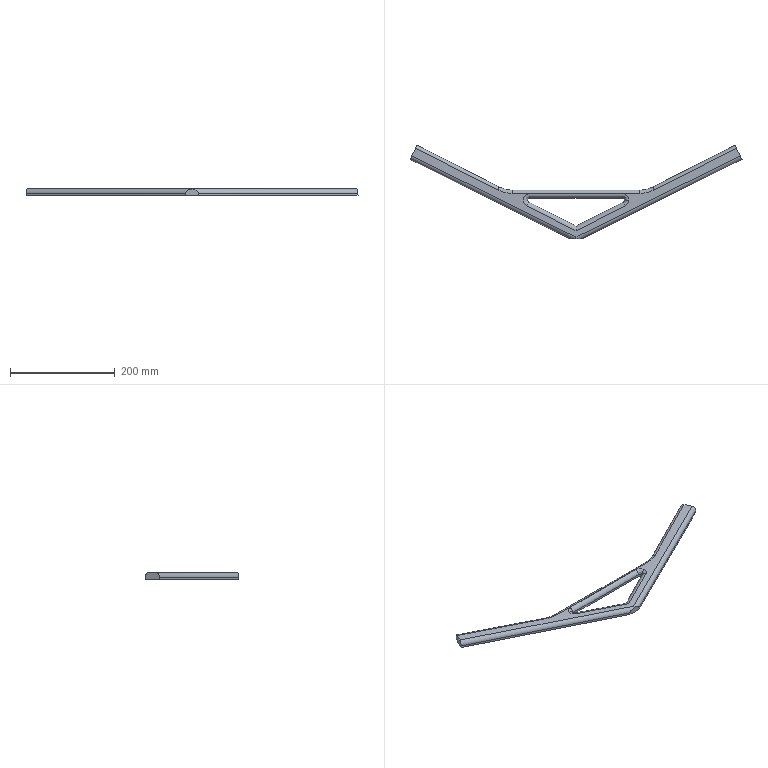Part | SolidWorks | features BaseBody 1 | 1 solid | 31 faces | box 633.433 x 177.606 x 12 mm | volume 259500 mm3 | cylinder 13 | plane 13 | spline 5 | commonest cylinder face diameters 16 x5 8 x3 12 x3 108 x2
STEP:
#1=CARTESIAN_POINT('',(-92.659,64.368,4.));
#2=VERTEX_POINT('',#1);
#3=CARTESIAN_POINT('',(-88.659,68.368,4.));
#4=VERTEX_POINT('',#3);
#5=CARTESIAN_POINT('',(-88.659,64.368,4.));
#6=DIRECTION('',(0.,0.,-1.));
#7=DIRECTION('',(-1.,0.,0.));
#8=AXIS2_PLACEMENT_3D('',#5,#6,#7);
#9=CIRCLE('',#8,4.);
#10=EDGE_CURVE('',#2,#4,#9,.T.);
#11=ORIENTED_EDGE('',*,*,#10,.F.);
#12=CARTESIAN_POINT('',(-92.659,64.368,0.));
#13=VERTEX_POINT('',#12);
#14=CARTESIAN_POINT('',(-92.659,64.368,4.));
#15=DIRECTION('',(0.,0.,-1.));
#16=VECTOR('',#15,1000.);
#17=LINE('',#14,#16);
#18=EDGE_CURVE('',#2,#13,#17,.T.);
#19=ORIENTED_EDGE('',*,*,#18,.T.);
#20=CARTESIAN_POINT('',(-88.659,68.368,0.));
#21=VERTEX_POINT('',#20);
#22=CARTESIAN_POINT('',(-88.659,64.368,0.));
#23=DIRECTION('',(0.,0.,-1.));
#24=DIRECTION('',(-1.,0.,0.));
#25=AXIS2_PLACEMENT_3D('',#22,#23,#24);
#26=CIRCLE('',#25,4.);
#27=EDGE_CURVE('',#13,#21,#26,.T.);
#28=ORIENTED_EDGE('',*,*,#27,.T.);
#29=CARTESIAN_POINT('',(-88.659,68.368,2.));
#30=DIRECTION('',(0.,0.,-1.));
#31=VECTOR('',#30,1000.);
#32=LINE('',#29,#31);
#33=EDGE_CURVE('',#4,#21,#32,.T.);
#34=ORIENTED_EDGE('',*,*,#33,.F.);
#35=EDGE_LOOP('',(#11,#19,#28,#34));
#36=FACE_OUTER_BOUND('',#35,.T.);
#37=CARTESIAN_POINT('',(-88.659,64.368,4.));
#38=DIRECTION('',(0.,0.,-1.));
#39=DIRECTION('',(-1.,0.,0.));
#40=AXIS2_PLACEMENT_3D('',#37,#38,#39);
#41=CYLINDRICAL_SURFACE('',#40,4.);
#42=ADVANCED_FACE('',(#36),#41,.F.);
#43=CARTESIAN_POINT('',(92.659,64.368,4.));
#44=VERTEX_POINT('',#43);
#45=CARTESIAN_POINT('',(90.467,60.8,4.));
#46=VERTEX_POINT('',#45);
#47=CARTESIAN_POINT('',(88.659,64.368,4.));
#48=DIRECTION('',(0.,0.,-1.));
#49=DIRECTION('',(-1.,0.,0.));
#50=AXIS2_PLACEMENT_3D('',#47,#48,#49);
#51=CIRCLE('',#50,4.);
#52=EDGE_CURVE('',#44,#46,#51,.T.);
#53=ORIENTED_EDGE('',*,*,#52,.T.);
#54=CARTESIAN_POINT('',(94.083,53.664,12.));
#55=VERTEX_POINT('',#54);
#56=CARTESIAN_POINT('',(94.083,53.664,4.));
#57=DIRECTION('',(0.892,0.452,0.));
#58=DIRECTION('',(-0.452,0.892,0.));
#59=AXIS2_PLACEMENT_3D('',#56,#57,#58);
#60=CIRCLE('',#59,8.);
#61=EDGE_CURVE('',#46,#55,#60,.T.);
#62=ORIENTED_EDGE('',*,*,#61,.T.);
#63=CARTESIAN_POINT('',(100.659,64.368,12.));
#64=VERTEX_POINT('',#63);
#65=CARTESIAN_POINT('',(94.083,53.664,12.));
#66=CARTESIAN_POINT('',(98.227,55.764,12.));
#67=CARTESIAN_POINT('',(100.659,59.722,12.));
#68=CARTESIAN_POINT('',(100.659,64.368,12.));
#69=(BOUNDED_CURVE()B_SPLINE_CURVE(3,(#65,#66,#67,#68),.UNSPECIFIED.,.F.,.F.)B_SPLINE_CURVE_WITH_KNOTS((4,4),(0.,1.),.UNSPECIFIED.)CURVE()GEOMETRIC_REPRESENTATION_ITEM()RATIONAL_B_SPLINE_CURVE((0.9566,0.8622,0.8622,0.9566))REPRESENTATION_ITEM(''));
#70=EDGE_CURVE('',#55,#64,#69,.T.);
#71=ORIENTED_EDGE('',*,*,#70,.T.);
#72=CARTESIAN_POINT('',(100.659,64.368,12.));
#73=CARTESIAN_POINT('',(95.973,64.368,12.));
#74=CARTESIAN_POINT('',(92.659,64.368,8.686));
#75=CARTESIAN_POINT('',(92.659,64.368,4.));
#76=(BOUNDED_CURVE()B_SPLINE_CURVE(3,(#72,#73,#74,#75),.UNSPECIFIED.,.F.,.F.)B_SPLINE_CURVE_WITH_KNOTS((4,4),(0.06314,0.9369),.UNSPECIFIED.)CURVE()GEOMETRIC_REPRESENTATION_ITEM()RATIONAL_B_SPLINE_CURVE((0.9566,0.7698,0.7698,0.9566))REPRESENTATION_ITEM(''));
#77=EDGE_CURVE('',#64,#44,#76,.T.);
#78=ORIENTED_EDGE('',*,*,#77,.T.);
#79=EDGE_LOOP('',(#53,#62,#71,#78));
#80=FACE_OUTER_BOUND('',#79,.T.);
#81=CARTESIAN_POINT('',(90.485,60.764,3.201));
#82=CARTESIAN_POINT('',(91.88,61.471,3.201));
#83=CARTESIAN_POINT('',(92.699,62.804,3.201));
#84=CARTESIAN_POINT('',(92.699,64.368,3.201));
#85=CARTESIAN_POINT('',(90.238,61.251,8.64));
#86=CARTESIAN_POINT('',(91.445,61.862,8.64));
#87=CARTESIAN_POINT('',(92.153,63.015,8.64));
#88=CARTESIAN_POINT('',(92.153,64.368,8.64));
#89=CARTESIAN_POINT('',(91.986,57.803,12.506));
#90=CARTESIAN_POINT('',(94.527,59.091,12.506));
#91=CARTESIAN_POINT('',(96.018,61.518,12.506));
#92=CARTESIAN_POINT('',(96.018,64.368,12.506));
#93=CARTESIAN_POINT('',(94.444,52.951,11.96));
#94=CARTESIAN_POINT('',(98.864,55.191,11.96));
#95=CARTESIAN_POINT('',(101.458,59.413,11.96));
#96=CARTESIAN_POINT('',(101.458,64.368,11.96));
#97=(BOUNDED_SURFACE()B_SPLINE_SURFACE(3,3,((#81,#82,#83,#84),(#85,#86,#87,#88),(#89,#90,#91,#92),(#93,#94,#95,#96)),.UNSPECIFIED.,.F.,.F.,.T.)B_SPLINE_SURFACE_WITH_KNOTS((4,4),(4,4),(0.,1.),(0.,1.),.UNSPECIFIED.)GEOMETRIC_REPRESENTATION_ITEM()RATIONAL_B_SPLINE_SURFACE(((1.,0.9014,0.9014,1.),(0.7553,0.6808,0.6808,0.7553),(0.7553,0.6808,0.6808,0.7553),(1.,0.9014,0.9014,1.)))REPRESENTATION_ITEM('')SURFACE());
#98=ADVANCED_FACE('',(#80),#97,.T.);
#99=CARTESIAN_POINT('',(0.,14.953,4.));
#100=VERTEX_POINT('',#99);
#101=CARTESIAN_POINT('',(43.143,36.817,4.));
#102=DIRECTION('',(0.892,0.452,0.));
#103=VECTOR('',#102,1000.);
#104=LINE('',#101,#103);
#105=EDGE_CURVE('',#100,#46,#104,.T.);
#106=ORIENTED_EDGE('',*,*,#105,.F.);
#107=CARTESIAN_POINT('',(0.000000027,5.985,12.));
#108=VERTEX_POINT('',#107);
#109=CARTESIAN_POINT('',(0.000000027,5.985,12.));
#110=CARTESIAN_POINT('',(0.,11.239,12.));
#111=CARTESIAN_POINT('',(0.,14.953,8.686));
#112=CARTESIAN_POINT('',(0.,14.953,4.));
#113=(BOUNDED_CURVE()B_SPLINE_CURVE(3,(#109,#110,#111,#112),.UNSPECIFIED.,.F.,.F.)B_SPLINE_CURVE_WITH_KNOTS((4,4),(4.712,6.283),.UNSPECIFIED.)CURVE()GEOMETRIC_REPRESENTATION_ITEM()RATIONAL_B_SPLINE_CURVE((1.,0.8047,0.8047,1.))REPRESENTATION_ITEM(''));
#114=EDGE_CURVE('',#108,#100,#113,.T.);
#115=ORIENTED_EDGE('',*,*,#114,.F.);
#116=CARTESIAN_POINT('',(46.759,29.681,12.));
#117=DIRECTION('',(-0.892,-0.452,0.));
#118=VECTOR('',#117,1000.);
#119=LINE('',#116,#118);
#120=EDGE_CURVE('',#55,#108,#119,.T.);
#121=ORIENTED_EDGE('',*,*,#120,.F.);
#122=ORIENTED_EDGE('',*,*,#61,.F.);
#123=EDGE_LOOP('',(#106,#115,#121,#122));
#124=FACE_OUTER_BOUND('',#123,.T.);
#125=CARTESIAN_POINT('',(-0.5645,5.699,4.));
#126=DIRECTION('',(0.892,0.452,0.));
#127=DIRECTION('',(-0.452,0.892,0.));
#128=AXIS2_PLACEMENT_3D('',#125,#126,#127);
#129=CYLINDRICAL_SURFACE('',#128,8.);
#130=ADVANCED_FACE('',(#124),#129,.T.);
#131=CARTESIAN_POINT('',(88.659,68.368,4.));
#132=VERTEX_POINT('',#131);
#133=CARTESIAN_POINT('',(88.659,68.368,0.));
#134=VERTEX_POINT('',#133);
#135=CARTESIAN_POINT('',(88.659,68.368,2.));
#136=DIRECTION('',(0.,0.,-1.));
#137=VECTOR('',#136,1000.);
#138=LINE('',#135,#137);
#139=EDGE_CURVE('',#132,#134,#138,.T.);
#140=ORIENTED_EDGE('',*,*,#139,.T.);
#141=CARTESIAN_POINT('',(90.467,60.8,0.));
#142=VERTEX_POINT('',#141);
#143=CARTESIAN_POINT('',(88.659,64.368,0.));
#144=DIRECTION('',(0.,0.,-1.));
#145=DIRECTION('',(-1.,0.,0.));
#146=AXIS2_PLACEMENT_3D('',#143,#144,#145);
#147=CIRCLE('',#146,4.);
#148=EDGE_CURVE('',#134,#142,#147,.T.);
#149=ORIENTED_EDGE('',*,*,#148,.T.);
#150=CARTESIAN_POINT('',(90.467,60.8,2.));
#151=DIRECTION('',(0.,0.,1.));
#152=VECTOR('',#151,1000.);
#153=LINE('',#150,#152);
#154=EDGE_CURVE('',#142,#46,#153,.T.);
#155=ORIENTED_EDGE('',*,*,#154,.T.);
#156=ORIENTED_EDGE('',*,*,#52,.F.);
#157=CARTESIAN_POINT('',(88.659,64.368,4.));
#158=DIRECTION('',(0.,0.,1.));
#159=DIRECTION('',(-1.,0.,0.));
#160=AXIS2_PLACEMENT_3D('',#157,#158,#159);
#161=CIRCLE('',#160,4.);
#162=EDGE_CURVE('',#44,#132,#161,.T.);
#163=ORIENTED_EDGE('',*,*,#162,.T.);
#164=EDGE_LOOP('',(#140,#149,#155,#156,#163));
#165=FACE_OUTER_BOUND('',#164,.T.);
#166=CARTESIAN_POINT('',(88.659,64.368,4.));
#167=DIRECTION('',(0.,0.,-1.));
#168=DIRECTION('',(-1.,0.,0.));
#169=AXIS2_PLACEMENT_3D('',#166,#167,#168);
#170=CYLINDRICAL_SURFACE('',#169,4.);
#171=ADVANCED_FACE('',(#165),#170,.F.);
#172=CARTESIAN_POINT('',(88.659,76.368,12.));
#173=VERTEX_POINT('',#172);
#174=CARTESIAN_POINT('',(88.659,76.368,4.));
#175=DIRECTION('',(1.,0.,0.));
#176=DIRECTION('',(0.,0.,-1.));
#177=AXIS2_PLACEMENT_3D('',#174,#175,#176);
#178=CIRCLE('',#177,8.);
#179=EDGE_CURVE('',#173,#132,#178,.T.);
#180=ORIENTED_EDGE('',*,*,#179,.T.);
#181=ORIENTED_EDGE('',*,*,#162,.F.);
#182=ORIENTED_EDGE('',*,*,#77,.F.);
#183=CARTESIAN_POINT('',(100.659,64.368,12.));
#184=CARTESIAN_POINT('',(100.659,71.397,12.));
#185=CARTESIAN_POINT('',(95.688,76.368,12.));
#186=CARTESIAN_POINT('',(88.659,76.368,12.));
#187=(BOUNDED_CURVE()B_SPLINE_CURVE(3,(#183,#184,#185,#186),.UNSPECIFIED.,.F.,.F.)B_SPLINE_CURVE_WITH_KNOTS((4,4),(0.,1.),.UNSPECIFIED.)CURVE()GEOMETRIC_REPRESENTATION_ITEM()RATIONAL_B_SPLINE_CURVE((0.9566,0.7698,0.7698,0.9566))REPRESENTATION_ITEM(''));
#188=EDGE_CURVE('',#64,#173,#187,.T.);
#189=ORIENTED_EDGE('',*,*,#188,.T.);
#190=EDGE_LOOP('',(#180,#181,#182,#189));
#191=FACE_OUTER_BOUND('',#190,.T.);
#192=CARTESIAN_POINT('',(92.699,64.368,3.201));
#193=CARTESIAN_POINT('',(92.699,66.734,3.201));
#194=CARTESIAN_POINT('',(91.025,68.408,3.201));
#195=CARTESIAN_POINT('',(88.659,68.408,3.201));
#196=CARTESIAN_POINT('',(92.153,64.368,8.64));
#197=CARTESIAN_POINT('',(92.153,66.414,8.64));
#198=CARTESIAN_POINT('',(90.706,67.862,8.64));
#199=CARTESIAN_POINT('',(88.659,67.862,8.64));
#200=CARTESIAN_POINT('',(96.018,64.368,12.506));
#201=CARTESIAN_POINT('',(96.018,68.679,12.506));
#202=CARTESIAN_POINT('',(92.97,71.727,12.506));
#203=CARTESIAN_POINT('',(88.659,71.727,12.506));
#204=CARTESIAN_POINT('',(101.458,64.368,11.96));
#205=CARTESIAN_POINT('',(101.458,71.865,11.96));
#206=CARTESIAN_POINT('',(96.156,77.166,11.96));
#207=CARTESIAN_POINT('',(88.659,77.166,11.96));
#208=(BOUNDED_SURFACE()B_SPLINE_SURFACE(3,3,((#192,#193,#194,#195),(#196,#197,#198,#199),(#200,#201,#202,#203),(#204,#205,#206,#207)),.UNSPECIFIED.,.F.,.F.,.F.)B_SPLINE_SURFACE_WITH_KNOTS((4,4),(4,4),(0.,1.),(0.,1.),.UNSPECIFIED.)GEOMETRIC_REPRESENTATION_ITEM()RATIONAL_B_SPLINE_SURFACE(((1.,0.8047,0.8047,1.),(0.7553,0.6078,0.6078,0.7553),(0.7553,0.6078,0.6078,0.7553),(1.,0.8047,0.8047,1.)))REPRESENTATION_ITEM('')SURFACE());
#209=ADVANCED_FACE('',(#191),#208,.T.);
#210=ORIENTED_EDGE('',*,*,#188,.F.);
#211=ORIENTED_EDGE('',*,*,#70,.F.);
#212=ORIENTED_EDGE('',*,*,#120,.T.);
#213=CARTESIAN_POINT('',(-94.083,53.664,12.));
#214=VERTEX_POINT('',#213);
#215=CARTESIAN_POINT('',(0.000000106,5.985,12.));
#216=DIRECTION('',(-0.892,0.452,0.));
#217=VECTOR('',#216,1000.);
#218=LINE('',#215,#217);
#219=EDGE_CURVE('',#108,#214,#218,.T.);
#220=ORIENTED_EDGE('',*,*,#219,.T.);
#221=CARTESIAN_POINT('',(-88.659,76.368,12.));
#222=VERTEX_POINT('',#221);
#223=CARTESIAN_POINT('',(-94.083,53.664,12.));
#224=CARTESIAN_POINT('',(-94.311,53.779,12.));
#225=CARTESIAN_POINT('',(-94.647,53.963,12.));
#226=CARTESIAN_POINT('',(-95.027,54.196,12.));
#227=CARTESIAN_POINT('',(-95.215,54.316,12.));
#228=CARTESIAN_POINT('',(-95.308,54.378,12.));
#229=CARTESIAN_POINT('',(-95.348,54.405,12.));
#230=CARTESIAN_POINT('',(-95.374,54.423,12.));
#231=CARTESIAN_POINT('',(-95.386,54.431,12.));
#232=CARTESIAN_POINT('',(-95.632,54.598,12.));
#233=CARTESIAN_POINT('',(-95.971,54.845,12.));
#234=CARTESIAN_POINT('',(-96.35,55.154,12.));
#235=CARTESIAN_POINT('',(-96.535,55.314,12.));
#236=CARTESIAN_POINT('',(-96.627,55.395,12.));
#237=CARTESIAN_POINT('',(-96.666,55.43,12.));
#238=CARTESIAN_POINT('',(-96.693,55.453,12.));
#239=CARTESIAN_POINT('',(-96.704,55.464,12.));
#240=CARTESIAN_POINT('',(-96.945,55.682,12.));
#241=CARTESIAN_POINT('',(-97.271,56.002,12.));
#242=CARTESIAN_POINT('',(-97.63,56.396,12.));
#243=CARTESIAN_POINT('',(-97.805,56.598,12.));
#244=CARTESIAN_POINT('',(-97.89,56.7,12.));
#245=CARTESIAN_POINT('',(-97.927,56.745,12.));
#246=CARTESIAN_POINT('',(-97.951,56.774,12.));
#247=CARTESIAN_POINT('',(-97.962,56.788,12.));
#248=CARTESIAN_POINT('',(-98.183,57.06,12.));
#249=CARTESIAN_POINT('',(-98.478,57.456,12.));
#250=CARTESIAN_POINT('',(-98.794,57.938,12.));
#251=CARTESIAN_POINT('',(-98.944,58.185,12.));
#252=CARTESIAN_POINT('',(-99.017,58.309,12.));
#253=CARTESIAN_POINT('',(-99.048,58.363,12.));
#254=CARTESIAN_POINT('',(-99.069,58.398,12.));
#255=CARTESIAN_POINT('',(-99.079,58.415,12.));
#256=CARTESIAN_POINT('',(-99.264,58.741,12.));
#257=CARTESIAN_POINT('',(-99.505,59.212,12.));
#258=CARTESIAN_POINT('',(-99.749,59.777,12.));
#259=CARTESIAN_POINT('',(-99.862,60.065,12.));
#260=CARTESIAN_POINT('',(-99.916,60.209,12.));
#261=CARTESIAN_POINT('',(-99.938,60.272,12.));
#262=CARTESIAN_POINT('',(-99.953,60.313,12.));
#263=CARTESIAN_POINT('',(-99.96,60.333,12.));
#264=CARTESIAN_POINT('',(-100.093,60.706,12.));
#265=CARTESIAN_POINT('',(-100.255,61.239,12.));
#266=CARTESIAN_POINT('',(-100.399,61.873,12.));
#267=CARTESIAN_POINT('',(-100.461,62.192,12.));
#268=CARTESIAN_POINT('',(-100.485,62.33,12.));
#269=CARTESIAN_POINT('',(-100.5,62.422,12.));
#270=CARTESIAN_POINT('',(-100.507,62.466,12.));
#271=CARTESIAN_POINT('',(-100.575,62.896,12.));
#272=CARTESIAN_POINT('',(-100.636,63.471,12.));
#273=CARTESIAN_POINT('',(-100.66,64.146,12.));
#274=CARTESIAN_POINT('',(-100.659,64.435,12.));
#275=CARTESIAN_POINT('',(-100.656,64.628,12.));
#276=CARTESIAN_POINT('',(-100.654,64.723,12.));
#277=CARTESIAN_POINT('',(-100.62,65.61,12.));
#278=CARTESIAN_POINT('',(-100.514,66.389,12.));
#279=CARTESIAN_POINT('',(-100.239,67.54,12.));
#280=CARTESIAN_POINT('',(-100.074,68.106,12.));
#281=CARTESIAN_POINT('',(-99.833,68.75,12.));
#282=CARTESIAN_POINT('',(-99.72,69.022,12.));
#283=CARTESIAN_POINT('',(-99.642,69.203,12.));
#284=CARTESIAN_POINT('',(-99.601,69.295,12.));
#285=CARTESIAN_POINT('',(-99.399,69.735,12.));
#286=CARTESIAN_POINT('',(-99.132,70.248,12.));
#287=CARTESIAN_POINT('',(-98.778,70.822,12.));
#288=CARTESIAN_POINT('',(-98.591,71.103,12.));
#289=CARTESIAN_POINT('',(-98.508,71.222,12.));
#290=CARTESIAN_POINT('',(-98.453,71.302,12.));
#291=CARTESIAN_POINT('',(-98.424,71.342,12.));
#292=CARTESIAN_POINT('',(-98.179,71.683,12.));
#293=CARTESIAN_POINT('',(-97.832,72.119,12.));
#294=CARTESIAN_POINT('',(-97.394,72.599,12.));
#295=CARTESIAN_POINT('',(-97.166,72.832,12.));
#296=CARTESIAN_POINT('',(-97.05,72.946,12.));
#297=CARTESIAN_POINT('',(-97.,72.995,12.));
#298=CARTESIAN_POINT('',(-96.966,73.027,12.));
#299=CARTESIAN_POINT('',(-96.949,73.044,12.));
#300=CARTESIAN_POINT('',(-96.677,73.303,12.));
#301=CARTESIAN_POINT('',(-96.279,73.65,12.));
#302=CARTESIAN_POINT('',(-95.788,74.023,12.));
#303=CARTESIAN_POINT('',(-95.537,74.202,12.));
#304=CARTESIAN_POINT('',(-95.409,74.289,12.));
#305=CARTESIAN_POINT('',(-95.354,74.326,12.));
#306=CARTESIAN_POINT('',(-95.318,74.351,12.));
#307=CARTESIAN_POINT('',(-95.298,74.364,12.));
#308=CARTESIAN_POINT('',(-95.006,74.557,12.));
#309=CARTESIAN_POINT('',(-94.583,74.813,12.));
#310=CARTESIAN_POINT('',(-94.072,75.08,12.));
#311=CARTESIAN_POINT('',(-93.812,75.205,12.));
#312=CARTESIAN_POINT('',(-93.681,75.266,12.));
#313=CARTESIAN_POINT('',(-93.625,75.292,12.));
#314=CARTESIAN_POINT('',(-93.587,75.309,12.));
#315=CARTESIAN_POINT('',(-93.567,75.318,12.));
#316=CARTESIAN_POINT('',(-93.271,75.45,12.));
#317=CARTESIAN_POINT('',(-92.847,75.62,12.));
#318=CARTESIAN_POINT('',(-92.341,75.79,12.));
#319=CARTESIAN_POINT('',(-92.086,75.868,12.));
#320=CARTESIAN_POINT('',(-91.958,75.905,12.));
#321=CARTESIAN_POINT('',(-91.903,75.921,12.));
#322=CARTESIAN_POINT('',(-91.866,75.931,12.));
#323=CARTESIAN_POINT('',(-91.846,75.937,12.));
#324=CARTESIAN_POINT('',(-91.559,76.015,12.));
#325=CARTESIAN_POINT('',(-91.151,76.112,12.));
#326=CARTESIAN_POINT('',(-90.67,76.199,12.));
#327=CARTESIAN_POINT('',(-90.428,76.237,12.));
#328=CARTESIAN_POINT('',(-90.307,76.254,12.));
#329=CARTESIAN_POINT('',(-90.255,76.261,12.));
#330=CARTESIAN_POINT('',(-90.22,76.266,12.));
#331=CARTESIAN_POINT('',(-90.201,76.268,12.));
#332=CARTESIAN_POINT('',(-89.679,76.335,12.));
#333=CARTESIAN_POINT('',(-89.17,76.367,12.));
#334=CARTESIAN_POINT('',(-88.659,76.368,12.));
#335=B_SPLINE_CURVE_WITH_KNOTS('',3,(#223,#224,#225,#226,#227,#228,#229,#230,#231,#232,#233,#234,#235,#236,#237,#238,#239,#240,#241,#242,#243,#244,#245,#246,#247,#248,#249,#250,#251,#252,#253,#254,#255,#256,#257,#258,#259,#260,#261,#262,#263,#264,#265,#266,#267,#268,#269,#270,#271,#272,#273,#274,#275,#276,#277,#278,#279,#280,#281,#282,#283,#284,#285,#286,#287,#288,#289,#290,#291,#292,#293,#294,#295,#296,#297,#298,#299,#300,#301,#302,#303,#304,#305,#306,#307,#308,#309,#310,#311,#312,#313,#314,#315,#316,#317,#318,#319,#320,#321,#322,#323,#324,#325,#326,#327,#328,#329,#330,#331,#332,#333,#334),.UNSPECIFIED.,.F.,.F.,(4,1,1,1,1,2,2,1,1,1,1,2,2,1,1,1,1,2,2,1,1,1,1,2,2,1,1,1,1,2,2,1,1,1,2,2,1,1,2,2,2,1,1,2,2,1,1,1,2,2,1,1,1,1,2,2,1,1,1,1,2,2,1,1,1,1,2,2,1,1,1,1,2,2,1,1,1,1,2,2,4),(0.,0.03125,0.04688,0.05469,0.05859,0.06055,0.0625,0.09375,0.1094,0.1172,0.1211,0.123,0.125,0.1563,0.1719,0.1797,0.1836,0.1855,0.1875,0.2188,0.2344,0.2422,0.2461,0.248,0.25,0.2813,0.2969,0.3047,0.3086,0.3105,0.3125,0.3438,0.3594,0.3672,0.3711,0.375,0.4063,0.4219,0.4297,0.4375,0.5,0.5313,0.5469,0.5547,0.5625,0.5938,0.6094,0.6172,0.6211,0.625,0.6563,0.6719,0.6797,0.6836,0.6855,0.6875,0.7188,0.7344,0.7422,0.7461,0.748,0.75,0.7813,0.7969,0.8047,0.8086,0.8105,0.8125,0.8438,0.8594,0.8672,0.8711,0.873,0.875,0.9063,0.9219,0.9297,0.9336,0.9355,0.9375,1.),.UNSPECIFIED.);
#336=EDGE_CURVE('',#214,#222,#335,.T.);
#337=ORIENTED_EDGE('',*,*,#336,.T.);
#338=CARTESIAN_POINT('',(0.,76.368,12.));
#339=DIRECTION('',(1.,0.,0.));
#340=VECTOR('',#339,1000.);
#341=LINE('',#338,#340);
#342=EDGE_CURVE('',#222,#173,#341,.T.);
#343=ORIENTED_EDGE('',*,*,#342,.T.);
#344=EDGE_LOOP('',(#210,#211,#212,#220,#337,#343));
#345=FACE_BOUND('',#344,.T.);
#346=CARTESIAN_POINT('',(-122.098,77.368,12.));
#347=VERTEX_POINT('',#346);
#348=CARTESIAN_POINT('',(-149.221,83.848,12.));
#349=VERTEX_POINT('',#348);
#350=CARTESIAN_POINT('',(-122.098,77.368,12.));
#351=CARTESIAN_POINT('',(-123.268,77.368,12.));
#352=CARTESIAN_POINT('',(-125.02,77.419,12.));
#353=CARTESIAN_POINT('',(-127.059,77.568,12.));
#354=CARTESIAN_POINT('',(-127.931,77.651,12.));
#355=CARTESIAN_POINT('',(-128.513,77.711,12.));
#356=CARTESIAN_POINT('',(-128.801,77.742,12.));
#357=CARTESIAN_POINT('',(-131.433,78.051,12.));
#358=CARTESIAN_POINT('',(-133.75,78.463,12.));
#359=CARTESIAN_POINT('',(-137.187,79.284,12.));
#360=CARTESIAN_POINT('',(-138.89,79.744,12.));
#361=CARTESIAN_POINT('',(-140.852,80.368,12.));
#362=CARTESIAN_POINT('',(-141.687,80.654,12.));
#363=CARTESIAN_POINT('',(-142.242,80.849,12.));
#364=CARTESIAN_POINT('',(-142.521,80.95,12.));
#365=CARTESIAN_POINT('',(-144.991,81.857,12.));
#366=CARTESIAN_POINT('',(-147.133,82.79,12.));
#367=CARTESIAN_POINT('',(-149.221,83.848,12.));
#368=B_SPLINE_CURVE_WITH_KNOTS('',3,(#350,#351,#352,#353,#354,#355,#356,#357,#358,#359,#360,#361,#362,#363,#364,#365,#366,#367),.UNSPECIFIED.,.F.,.F.,(4,1,1,2,2,2,1,1,2,2,4),(0.,0.125,0.1875,0.2187,0.25,0.5,0.625,0.6875,0.7187,0.75,1.),.UNSPECIFIED.);
#369=EDGE_CURVE('',#347,#349,#368,.T.);
#370=ORIENTED_EDGE('',*,*,#369,.T.);
#371=CARTESIAN_POINT('',(-305.97,163.284,12.));
#372=VERTEX_POINT('',#371);
#373=CARTESIAN_POINT('',(-149.221,83.848,12.));
#374=DIRECTION('',(-0.892,0.452,0.));
#375=VECTOR('',#374,1000.);
#376=LINE('',#373,#375);
#377=EDGE_CURVE('',#349,#372,#376,.T.);
#378=ORIENTED_EDGE('',*,*,#377,.T.);
#379=CARTESIAN_POINT('',(-313.134,148.977,12.));
#380=VERTEX_POINT('',#379);
#381=CARTESIAN_POINT('',(-305.97,163.284,12.));
#382=DIRECTION('',(-0.4478,-0.8942,0.));
#383=VECTOR('',#382,1000.);
#384=LINE('',#381,#383);
#385=EDGE_CURVE('',#372,#380,#384,.T.);
#386=ORIENTED_EDGE('',*,*,#385,.T.);
#387=CARTESIAN_POINT('',(0.,-5.956,12.));
#388=VERTEX_POINT('',#387);
#389=CARTESIAN_POINT('',(-313.134,148.977,12.));
#390=DIRECTION('',(0.8963,-0.4435,0.));
#391=VECTOR('',#390,1000.);
#392=LINE('',#389,#391);
#393=EDGE_CURVE('',#380,#388,#392,.T.);
#394=ORIENTED_EDGE('',*,*,#393,.T.);
#395=CARTESIAN_POINT('',(313.134,148.977,12.));
#396=VERTEX_POINT('',#395);
#397=CARTESIAN_POINT('',(0.,-5.956,12.));
#398=DIRECTION('',(0.8963,0.4435,0.));
#399=VECTOR('',#398,1000.);
#400=LINE('',#397,#399);
#401=EDGE_CURVE('',#388,#396,#400,.T.);
#402=ORIENTED_EDGE('',*,*,#401,.T.);
#403=CARTESIAN_POINT('',(305.97,163.284,12.));
#404=VERTEX_POINT('',#403);
#405=CARTESIAN_POINT('',(313.134,148.977,12.));
#406=DIRECTION('',(-0.4478,0.8942,0.));
#407=VECTOR('',#406,1000.);
#408=LINE('',#405,#407);
#409=EDGE_CURVE('',#396,#404,#408,.T.);
#410=ORIENTED_EDGE('',*,*,#409,.T.);
#411=CARTESIAN_POINT('',(149.221,83.848,12.));
#412=VERTEX_POINT('',#411);
#413=CARTESIAN_POINT('',(305.97,163.284,12.));
#414=DIRECTION('',(-0.892,-0.452,0.));
#415=VECTOR('',#414,1000.);
#416=LINE('',#413,#415);
#417=EDGE_CURVE('',#404,#412,#416,.T.);
#418=ORIENTED_EDGE('',*,*,#417,.T.);
#419=CARTESIAN_POINT('',(122.098,77.368,12.));
#420=VERTEX_POINT('',#419);
#421=CARTESIAN_POINT('',(149.221,83.848,12.));
#422=CARTESIAN_POINT('',(148.177,83.319,12.));
#423=CARTESIAN_POINT('',(146.591,82.572,12.));
#424=CARTESIAN_POINT('',(144.705,81.784,12.));
#425=CARTESIAN_POINT('',(143.889,81.464,12.));
#426=CARTESIAN_POINT('',(143.344,81.254,12.));
#427=CARTESIAN_POINT('',(143.072,81.152,12.));
#428=CARTESIAN_POINT('',(140.585,80.238,12.));
#429=CARTESIAN_POINT('',(138.332,79.557,12.));
#430=CARTESIAN_POINT('',(134.895,78.736,12.));
#431=CARTESIAN_POINT('',(133.168,78.377,12.));
#432=CARTESIAN_POINT('',(131.136,78.047,12.));
#433=CARTESIAN_POINT('',(130.262,77.925,12.));
#434=CARTESIAN_POINT('',(129.678,77.848,12.));
#435=CARTESIAN_POINT('',(129.384,77.811,12.));
#436=CARTESIAN_POINT('',(126.77,77.504,12.));
#437=CARTESIAN_POINT('',(124.439,77.368,12.));
#438=CARTESIAN_POINT('',(122.098,77.368,12.));
#439=B_SPLINE_CURVE_WITH_KNOTS('',3,(#421,#422,#423,#424,#425,#426,#427,#428,#429,#430,#431,#432,#433,#434,#435,#436,#437,#438),.UNSPECIFIED.,.F.,.F.,(4,1,1,2,2,2,1,1,2,2,4),(0.,0.125,0.1875,0.2187,0.25,0.5,0.625,0.6875,0.7187,0.75,1.),.UNSPECIFIED.);
#440=EDGE_CURVE('',#412,#420,#439,.T.);
#441=ORIENTED_EDGE('',*,*,#440,.T.);
#442=CARTESIAN_POINT('',(0.,77.368,12.));
#443=DIRECTION('',(-1.,0.,0.));
#444=VECTOR('',#443,1000.);
#445=LINE('',#442,#444);
#446=EDGE_CURVE('',#420,#347,#445,.T.);
#447=ORIENTED_EDGE('',*,*,#446,.T.);
#448=EDGE_LOOP('',(#370,#378,#386,#394,#402,#410,#418,#441,#447));
#449=FACE_OUTER_BOUND('',#448,.T.);
#450=CARTESIAN_POINT('',(-316.892,-6.972,12.));
#451=DIRECTION('',(0.,0.,1.));
#452=DIRECTION('',(1.,0.,0.));
#453=AXIS2_PLACEMENT_3D('',#450,#451,#452);
#454=PLANE('',#453);
#455=ADVANCED_FACE('',(#345,#449),#454,.T.);
#456=ORIENTED_EDGE('',*,*,#154,.F.);
#457=CARTESIAN_POINT('',(0.,14.953,0.));
#458=VERTEX_POINT('',#457);
#459=CARTESIAN_POINT('',(45.234,37.877,0.));
#460=DIRECTION('',(-0.892,-0.452,0.));
#461=VECTOR('',#460,1000.);
#462=LINE('',#459,#461);
#463=EDGE_CURVE('',#142,#458,#462,.T.);
#464=ORIENTED_EDGE('',*,*,#463,.T.);
#465=CARTESIAN_POINT('',(0.,14.953,2.));
#466=DIRECTION('',(0.,0.,1.));
#467=VECTOR('',#466,1000.);
#468=LINE('',#465,#467);
#469=EDGE_CURVE('',#458,#100,#468,.T.);
#470=ORIENTED_EDGE('',*,*,#469,.T.);
#471=ORIENTED_EDGE('',*,*,#105,.T.);
#472=EDGE_LOOP('',(#456,#464,#470,#471));
#473=FACE_OUTER_BOUND('',#472,.T.);
#474=CARTESIAN_POINT('',(90.467,60.8,0.));
#475=DIRECTION('',(-0.452,0.892,0.));
#476=DIRECTION('',(-0.892,-0.452,0.));
#477=AXIS2_PLACEMENT_3D('',#474,#475,#476);
#478=PLANE('',#477);
#479=ADVANCED_FACE('',(#473),#478,.T.);
#480=ORIENTED_EDGE('',*,*,#219,.F.);
#481=ORIENTED_EDGE('',*,*,#114,.T.);
#482=CARTESIAN_POINT('',(-90.467,60.8,4.));
#483=VERTEX_POINT('',#482);
#484=CARTESIAN_POINT('',(-43.143,36.817,4.));
#485=DIRECTION('',(0.892,-0.452,0.));
#486=VECTOR('',#485,1000.);
#487=LINE('',#484,#486);
#488=EDGE_CURVE('',#483,#100,#487,.T.);
#489=ORIENTED_EDGE('',*,*,#488,.F.);
#490=CARTESIAN_POINT('',(-94.083,53.664,4.));
#491=DIRECTION('',(-0.892,0.452,0.));
#492=DIRECTION('',(0.452,0.892,0.));
#493=AXIS2_PLACEMENT_3D('',#490,#491,#492);
#494=CIRCLE('',#493,8.);
#495=EDGE_CURVE('',#214,#483,#494,.T.);
#496=ORIENTED_EDGE('',*,*,#495,.F.);
#497=EDGE_LOOP('',(#480,#481,#489,#496));
#498=FACE_OUTER_BOUND('',#497,.T.);
#499=CARTESIAN_POINT('',(-94.083,53.664,4.));
#500=DIRECTION('',(0.892,-0.452,0.));
#501=DIRECTION('',(0.452,0.892,0.));
#502=AXIS2_PLACEMENT_3D('',#499,#500,#501);
#503=CYLINDRICAL_SURFACE('',#502,8.);
#504=ADVANCED_FACE('',(#498),#503,.T.);
#505=CARTESIAN_POINT('',(0.,68.368,0.));
#506=DIRECTION('',(1.,0.,0.));
#507=VECTOR('',#506,1000.);
#508=LINE('',#505,#507);
#509=EDGE_CURVE('',#21,#134,#508,.T.);
#510=ORIENTED_EDGE('',*,*,#509,.F.);
#511=ORIENTED_EDGE('',*,*,#27,.F.);
#512=CARTESIAN_POINT('',(-90.467,60.8,0.));
#513=VERTEX_POINT('',#512);
#514=CARTESIAN_POINT('',(-88.659,64.368,0.));
#515=DIRECTION('',(0.,0.,-1.));
#516=DIRECTION('',(-1.,0.,0.));
#517=AXIS2_PLACEMENT_3D('',#514,#515,#516);
#518=CIRCLE('',#517,4.);
#519=EDGE_CURVE('',#513,#13,#518,.T.);
#520=ORIENTED_EDGE('',*,*,#519,.F.);
#521=CARTESIAN_POINT('',(0.,14.953,0.));
#522=DIRECTION('',(-0.892,0.452,0.));
#523=VECTOR('',#522,1000.);
#524=LINE('',#521,#523);
#525=EDGE_CURVE('',#458,#513,#524,.T.);
#526=ORIENTED_EDGE('',*,*,#525,.F.);
#527=ORIENTED_EDGE('',*,*,#463,.F.);
#528=ORIENTED_EDGE('',*,*,#148,.F.);
#529=EDGE_LOOP('',(#510,#511,#520,#526,#527,#528));
#530=FACE_BOUND('',#529,.T.);
#531=CARTESIAN_POINT('',(-303.284,168.649,0.));
#532=VERTEX_POINT('',#531);
#533=CARTESIAN_POINT('',(-316.716,141.824,0.));
#534=VERTEX_POINT('',#533);
#535=CARTESIAN_POINT('',(-316.716,141.824,0.));
#536=DIRECTION('',(-0.4478,-0.8942,0.));
#537=VECTOR('',#536,1000.);
#538=LINE('',#535,#537);
#539=EDGE_CURVE('',#532,#534,#538,.T.);
#540=ORIENTED_EDGE('',*,*,#539,.F.);
#541=CARTESIAN_POINT('',(-146.508,89.2,0.));
#542=VERTEX_POINT('',#541);
#543=CARTESIAN_POINT('',(-303.284,168.649,0.));
#544=DIRECTION('',(-0.892,0.452,0.));
#545=VECTOR('',#544,1000.);
#546=LINE('',#543,#545);
#547=EDGE_CURVE('',#542,#532,#546,.T.);
#548=ORIENTED_EDGE('',*,*,#547,.F.);
#549=CARTESIAN_POINT('',(-122.098,83.368,0.));
#550=VERTEX_POINT('',#549);
#551=CARTESIAN_POINT('',(-122.098,137.368,0.));
#552=DIRECTION('',(0.,0.,-1.));
#553=DIRECTION('',(-1.,0.,0.));
#554=AXIS2_PLACEMENT_3D('',#551,#552,#553);
#555=CIRCLE('',#554,54.);
#556=EDGE_CURVE('',#550,#542,#555,.T.);
#557=ORIENTED_EDGE('',*,*,#556,.F.);
#558=CARTESIAN_POINT('',(122.098,83.368,0.));
#559=VERTEX_POINT('',#558);
#560=CARTESIAN_POINT('',(0.,83.368,0.));
#561=DIRECTION('',(-1.,0.,0.));
#562=VECTOR('',#561,1000.);
#563=LINE('',#560,#562);
#564=EDGE_CURVE('',#559,#550,#563,.T.);
#565=ORIENTED_EDGE('',*,*,#564,.F.);
#566=CARTESIAN_POINT('',(146.508,89.2,0.000000001));
#567=VERTEX_POINT('',#566);
#568=CARTESIAN_POINT('',(122.098,137.368,0.));
#569=DIRECTION('',(0.,0.,-1.));
#570=DIRECTION('',(-1.,0.,0.));
#571=AXIS2_PLACEMENT_3D('',#568,#569,#570);
#572=CIRCLE('',#571,54.);
#573=EDGE_CURVE('',#567,#559,#572,.T.);
#574=ORIENTED_EDGE('',*,*,#573,.F.);
#575=CARTESIAN_POINT('',(303.284,168.649,0.000000013));
#576=VERTEX_POINT('',#575);
#577=CARTESIAN_POINT('',(146.508,89.2,0.000000002));
#578=DIRECTION('',(-0.892,-0.452,0.));
#579=VECTOR('',#578,1000.);
#580=LINE('',#577,#579);
#581=EDGE_CURVE('',#576,#567,#580,.T.);
#582=ORIENTED_EDGE('',*,*,#581,.F.);
#583=CARTESIAN_POINT('',(316.716,141.824,0.000000012));
#584=VERTEX_POINT('',#583);
#585=CARTESIAN_POINT('',(303.284,168.649,0.000000023));
#586=DIRECTION('',(-0.4478,0.8942,0.));
#587=VECTOR('',#586,1000.);
#588=LINE('',#585,#587);
#589=EDGE_CURVE('',#584,#576,#588,.T.);
#590=ORIENTED_EDGE('',*,*,#589,.F.);
#591=CARTESIAN_POINT('',(11.974,-8.957,0.));
#592=VERTEX_POINT('',#591);
#593=CARTESIAN_POINT('',(316.716,141.824,0.));
#594=DIRECTION('',(0.8963,0.4435,0.));
#595=VECTOR('',#594,1000.);
#596=LINE('',#593,#595);
#597=EDGE_CURVE('',#592,#584,#596,.T.);
#598=ORIENTED_EDGE('',*,*,#597,.F.);
#599=CARTESIAN_POINT('',(-11.974,-8.957,0.));
#600=VERTEX_POINT('',#599);
#601=CARTESIAN_POINT('',(0.,-8.957,0.));
#602=DIRECTION('',(1.,0.,0.));
#603=VECTOR('',#602,1000.);
#604=LINE('',#601,#603);
#605=EDGE_CURVE('',#600,#592,#604,.T.);
#606=ORIENTED_EDGE('',*,*,#605,.F.);
#607=CARTESIAN_POINT('',(-11.974,-8.957,0.));
#608=DIRECTION('',(0.8963,-0.4435,0.));
#609=VECTOR('',#608,1000.);
#610=LINE('',#607,#609);
#611=EDGE_CURVE('',#534,#600,#610,.T.);
#612=ORIENTED_EDGE('',*,*,#611,.F.);
#613=EDGE_LOOP('',(#540,#548,#557,#565,#574,#582,#590,#598,#606,#612));
#614=FACE_OUTER_BOUND('',#613,.T.);
#615=CARTESIAN_POINT('',(-320.517,-8.957,0.));
#616=DIRECTION('',(0.,0.,1.));
#617=DIRECTION('',(1.,0.,0.));
#618=AXIS2_PLACEMENT_3D('',#615,#616,#617);
#619=PLANE('',#618);
#620=ADVANCED_FACE('',(#530,#614),#619,.F.);
#621=ORIENTED_EDGE('',*,*,#33,.T.);
#622=ORIENTED_EDGE('',*,*,#509,.T.);
#623=ORIENTED_EDGE('',*,*,#139,.F.);
#624=CARTESIAN_POINT('',(0.,68.368,4.));
#625=DIRECTION('',(-1.,0.,0.));
#626=VECTOR('',#625,1000.);
#627=LINE('',#624,#626);
#628=EDGE_CURVE('',#132,#4,#627,.T.);
#629=ORIENTED_EDGE('',*,*,#628,.T.);
#630=EDGE_LOOP('',(#621,#622,#623,#629));
#631=FACE_OUTER_BOUND('',#630,.T.);
#632=CARTESIAN_POINT('',(-88.659,68.368,4.));
#633=DIRECTION('',(0.,-1.,0.));
#634=DIRECTION('',(0.,0.,-1.));
#635=AXIS2_PLACEMENT_3D('',#632,#633,#634);
#636=PLANE('',#635);
#637=ADVANCED_FACE('',(#631),#636,.T.);
#638=ORIENTED_EDGE('',*,*,#628,.F.);
#639=ORIENTED_EDGE('',*,*,#179,.F.);
#640=ORIENTED_EDGE('',*,*,#342,.F.);
#641=CARTESIAN_POINT('',(-88.659,76.368,4.));
#642=DIRECTION('',(-1.,0.,0.));
#643=DIRECTION('',(0.,0.,1.));
#644=AXIS2_PLACEMENT_3D('',#641,#642,#643);
#645=CIRCLE('',#644,8.);
#646=EDGE_CURVE('',#4,#222,#645,.T.);
#647=ORIENTED_EDGE('',*,*,#646,.F.);
#648=EDGE_LOOP('',(#638,#639,#640,#647));
#649=FACE_OUTER_BOUND('',#648,.T.);
#650=CARTESIAN_POINT('',(88.659,76.368,4.));
#651=DIRECTION('',(-1.,0.,0.));
#652=DIRECTION('',(0.,0.,1.));
#653=AXIS2_PLACEMENT_3D('',#650,#651,#652);
#654=CYLINDRICAL_SURFACE('',#653,8.);
#655=ADVANCED_FACE('',(#649),#654,.T.);
#656=ORIENTED_EDGE('',*,*,#495,.T.);
#657=CARTESIAN_POINT('',(-88.659,64.368,4.));
#658=DIRECTION('',(0.,0.,-1.));
#659=DIRECTION('',(-1.,0.,0.));
#660=AXIS2_PLACEMENT_3D('',#657,#658,#659);
#661=CIRCLE('',#660,4.);
#662=EDGE_CURVE('',#483,#2,#661,.T.);
#663=ORIENTED_EDGE('',*,*,#662,.T.);
#664=ORIENTED_EDGE('',*,*,#10,.T.);
#665=ORIENTED_EDGE('',*,*,#646,.T.);
#666=ORIENTED_EDGE('',*,*,#336,.F.);
#667=EDGE_LOOP('',(#656,#663,#664,#665,#666));
#668=FACE_OUTER_BOUND('',#667,.T.);
#669=CARTESIAN_POINT('',(-88.659,68.408,3.201));
#670=CARTESIAN_POINT('',(-94.024,68.408,3.201));
#671=CARTESIAN_POINT('',(-95.271,63.189,3.201));
#672=CARTESIAN_POINT('',(-90.485,60.764,3.201));
#673=CARTESIAN_POINT('',(-88.659,67.862,8.64));
#674=CARTESIAN_POINT('',(-93.299,67.862,8.64));
#675=CARTESIAN_POINT('',(-94.378,63.348,8.64));
#676=CARTESIAN_POINT('',(-90.238,61.251,8.64));
#677=CARTESIAN_POINT('',(-88.659,71.727,12.506));
#678=CARTESIAN_POINT('',(-98.433,71.727,12.506));
#679=CARTESIAN_POINT('',(-100.704,62.221,12.506));
#680=CARTESIAN_POINT('',(-91.986,57.803,12.506));
#681=CARTESIAN_POINT('',(-88.659,77.166,11.96));
#682=CARTESIAN_POINT('',(-105.656,77.166,11.96));
#683=CARTESIAN_POINT('',(-109.606,60.634,11.96));
#684=CARTESIAN_POINT('',(-94.444,52.951,11.96));
#685=(BOUNDED_SURFACE()B_SPLINE_SURFACE(3,3,((#669,#670,#671,#672),(#673,#674,#675,#676),(#677,#678,#679,#680),(#681,#682,#683,#684)),.UNSPECIFIED.,.F.,.F.,.T.)B_SPLINE_SURFACE_WITH_KNOTS((4,4),(4,4),(0.,1.),(0.,1.),.UNSPECIFIED.)GEOMETRIC_REPRESENTATION_ITEM()RATIONAL_B_SPLINE_SURFACE(((1.,0.4883,0.4883,1.),(0.7553,0.3688,0.3688,0.7553),(0.7553,0.3688,0.3688,0.7553),(1.,0.4883,0.4883,1.)))REPRESENTATION_ITEM('')SURFACE());
#686=ADVANCED_FACE('',(#668),#685,.T.);
#687=CARTESIAN_POINT('',(-303.284,168.649,6.));
#688=VERTEX_POINT('',#687);
#689=CARTESIAN_POINT('',(-146.508,89.2,6.));
#690=VERTEX_POINT('',#689);
#691=CARTESIAN_POINT('',(-225.366,129.163,6.));
#692=DIRECTION('',(0.892,-0.452,0.));
#693=VECTOR('',#692,1000.);
#694=LINE('',#691,#693);
#695=EDGE_CURVE('',#688,#690,#694,.T.);
#696=ORIENTED_EDGE('',*,*,#695,.F.);
#697=CARTESIAN_POINT('',(-305.97,163.284,12.));
#698=CARTESIAN_POINT('',(-304.396,166.426,12.));
#699=CARTESIAN_POINT('',(-303.284,168.649,9.515));
#700=CARTESIAN_POINT('',(-303.284,168.649,6.));
#701=(BOUNDED_CURVE()B_SPLINE_CURVE(3,(#697,#698,#699,#700),.UNSPECIFIED.,.F.,.F.)B_SPLINE_CURVE_WITH_KNOTS((4,4),(1.571,3.142),.UNSPECIFIED.)CURVE()GEOMETRIC_REPRESENTATION_ITEM()RATIONAL_B_SPLINE_CURVE((1.,0.8047,0.8047,1.))REPRESENTATION_ITEM(''));
#702=EDGE_CURVE('',#372,#688,#701,.T.);
#703=ORIENTED_EDGE('',*,*,#702,.F.);
#704=ORIENTED_EDGE('',*,*,#377,.F.);
#705=CARTESIAN_POINT('',(-149.221,83.848,6.));
#706=DIRECTION('',(0.892,-0.452,0.));
#707=DIRECTION('',(0.452,0.892,0.));
#708=AXIS2_PLACEMENT_3D('',#705,#706,#707);
#709=CIRCLE('',#708,6.);
#710=EDGE_CURVE('',#690,#349,#709,.T.);
#711=ORIENTED_EDGE('',*,*,#710,.F.);
#712=EDGE_LOOP('',(#696,#703,#704,#711));
#713=FACE_OUTER_BOUND('',#712,.T.);
#714=CARTESIAN_POINT('',(-306.936,163.773,6.));
#715=DIRECTION('',(0.892,-0.452,0.));
#716=DIRECTION('',(0.452,0.892,0.));
#717=AXIS2_PLACEMENT_3D('',#714,#715,#716);
#718=CYLINDRICAL_SURFACE('',#717,6.);
#719=ADVANCED_FACE('',(#713),#718,.T.);
#720=ORIENTED_EDGE('',*,*,#710,.T.);
#721=ORIENTED_EDGE('',*,*,#369,.F.);
#722=CARTESIAN_POINT('',(-122.098,83.368,6.));
#723=VERTEX_POINT('',#722);
#724=CARTESIAN_POINT('',(-122.098,77.368,6.));
#725=DIRECTION('',(-1.,0.,0.));
#726=DIRECTION('',(0.,0.,-1.));
#727=AXIS2_PLACEMENT_3D('',#724,#725,#726);
#728=CIRCLE('',#727,6.);
#729=EDGE_CURVE('',#347,#723,#728,.T.);
#730=ORIENTED_EDGE('',*,*,#729,.T.);
#731=CARTESIAN_POINT('',(-122.098,137.368,6.));
#732=DIRECTION('',(0.,0.,-1.));
#733=DIRECTION('',(0.,1.,0.));
#734=AXIS2_PLACEMENT_3D('',#731,#732,#733);
#735=CIRCLE('',#734,54.);
#736=EDGE_CURVE('',#723,#690,#735,.T.);
#737=ORIENTED_EDGE('',*,*,#736,.T.);
#738=EDGE_LOOP('',(#720,#721,#730,#737));
#739=FACE_OUTER_BOUND('',#738,.T.);
#740=CARTESIAN_POINT('',(-146.522,89.173,5.401));
#741=CARTESIAN_POINT('',(-138.917,85.319,5.401));
#742=CARTESIAN_POINT('',(-130.624,83.338,5.401));
#743=CARTESIAN_POINT('',(-122.098,83.338,5.401));
#744=CARTESIAN_POINT('',(-146.337,89.538,9.48));
#745=CARTESIAN_POINT('',(-138.789,85.713,9.48));
#746=CARTESIAN_POINT('',(-130.56,83.747,9.48));
#747=CARTESIAN_POINT('',(-122.098,83.747,9.48));
#748=CARTESIAN_POINT('',(-147.647,86.952,12.379));
#749=CARTESIAN_POINT('',(-139.692,82.92,12.379));
#750=CARTESIAN_POINT('',(-131.017,80.848,12.379));
#751=CARTESIAN_POINT('',(-122.098,80.848,12.379));
#752=CARTESIAN_POINT('',(-149.491,83.313,11.97));
#753=CARTESIAN_POINT('',(-140.962,78.991,11.97));
#754=CARTESIAN_POINT('',(-131.661,76.769,11.97));
#755=CARTESIAN_POINT('',(-122.098,76.769,11.97));
#756=(BOUNDED_SURFACE()B_SPLINE_SURFACE(3,3,((#740,#741,#742,#743),(#744,#745,#746,#747),(#748,#749,#750,#751),(#752,#753,#754,#755)),.UNSPECIFIED.,.F.,.F.,.F.)B_SPLINE_SURFACE_WITH_KNOTS((4,4),(4,4),(0.,1.),(0.,1.),.UNSPECIFIED.)GEOMETRIC_REPRESENTATION_ITEM()RATIONAL_B_SPLINE_SURFACE(((1.,0.9817,0.9817,1.),(0.7553,0.7415,0.7415,0.7553),(0.7553,0.7415,0.7415,0.7553),(1.,0.9817,0.9817,1.)))REPRESENTATION_ITEM('')SURFACE());
#757=ADVANCED_FACE('',(#739),#756,.T.);
#758=CARTESIAN_POINT('',(122.098,83.368,6.));
#759=VERTEX_POINT('',#758);
#760=CARTESIAN_POINT('',(0.,83.368,6.));
#761=DIRECTION('',(1.,0.,0.));
#762=VECTOR('',#761,1000.);
#763=LINE('',#760,#762);
#764=EDGE_CURVE('',#723,#759,#763,.T.);
#765=ORIENTED_EDGE('',*,*,#764,.F.);
#766=ORIENTED_EDGE('',*,*,#729,.F.);
#767=ORIENTED_EDGE('',*,*,#446,.F.);
#768=CARTESIAN_POINT('',(122.098,77.368,6.));
#769=DIRECTION('',(1.,0.,0.));
#770=DIRECTION('',(0.,1.,0.));
#771=AXIS2_PLACEMENT_3D('',#768,#769,#770);
#772=CIRCLE('',#771,6.);
#773=EDGE_CURVE('',#759,#420,#772,.T.);
#774=ORIENTED_EDGE('',*,*,#773,.F.);
#775=EDGE_LOOP('',(#765,#766,#767,#774));
#776=FACE_OUTER_BOUND('',#775,.T.);
#777=CARTESIAN_POINT('',(-122.098,77.368,6.));
#778=DIRECTION('',(1.,0.,0.));
#779=DIRECTION('',(0.,0.,-1.));
#780=AXIS2_PLACEMENT_3D('',#777,#778,#779);
#781=CYLINDRICAL_SURFACE('',#780,6.);
#782=ADVANCED_FACE('',(#776),#781,.T.);
#783=ORIENTED_EDGE('',*,*,#773,.T.);
#784=ORIENTED_EDGE('',*,*,#440,.F.);
#785=CARTESIAN_POINT('',(146.508,89.2,6.));
#786=VERTEX_POINT('',#785);
#787=CARTESIAN_POINT('',(149.221,83.848,6.));
#788=DIRECTION('',(-0.892,-0.452,0.));
#789=DIRECTION('',(-0.452,0.892,0.));
#790=AXIS2_PLACEMENT_3D('',#787,#788,#789);
#791=CIRCLE('',#790,6.);
#792=EDGE_CURVE('',#412,#786,#791,.T.);
#793=ORIENTED_EDGE('',*,*,#792,.T.);
#794=CARTESIAN_POINT('',(122.098,137.368,6.));
#795=DIRECTION('',(0.,0.,-1.));
#796=DIRECTION('',(-1.,0.,0.));
#797=AXIS2_PLACEMENT_3D('',#794,#795,#796);
#798=CIRCLE('',#797,54.);
#799=EDGE_CURVE('',#786,#759,#798,.T.);
#800=ORIENTED_EDGE('',*,*,#799,.T.);
#801=EDGE_LOOP('',(#783,#784,#793,#800));
#802=FACE_OUTER_BOUND('',#801,.T.);
#803=CARTESIAN_POINT('',(122.098,83.338,5.401));
#804=CARTESIAN_POINT('',(130.624,83.338,5.401));
#805=CARTESIAN_POINT('',(138.917,85.319,5.401));
#806=CARTESIAN_POINT('',(146.522,89.173,5.401));
#807=CARTESIAN_POINT('',(122.098,83.747,9.48));
#808=CARTESIAN_POINT('',(130.56,83.747,9.48));
#809=CARTESIAN_POINT('',(138.789,85.713,9.48));
#810=CARTESIAN_POINT('',(146.337,89.538,9.48));
#811=CARTESIAN_POINT('',(122.098,80.848,12.379));
#812=CARTESIAN_POINT('',(131.017,80.848,12.379));
#813=CARTESIAN_POINT('',(139.692,82.92,12.379));
#814=CARTESIAN_POINT('',(147.647,86.952,12.379));
#815=CARTESIAN_POINT('',(122.098,76.769,11.97));
#816=CARTESIAN_POINT('',(131.661,76.769,11.97));
#817=CARTESIAN_POINT('',(140.962,78.991,11.97));
#818=CARTESIAN_POINT('',(149.491,83.313,11.97));
#819=(BOUNDED_SURFACE()B_SPLINE_SURFACE(3,3,((#803,#804,#805,#806),(#807,#808,#809,#810),(#811,#812,#813,#814),(#815,#816,#817,#818)),.UNSPECIFIED.,.F.,.F.,.T.)B_SPLINE_SURFACE_WITH_KNOTS((4,4),(4,4),(0.,1.),(0.,1.),.UNSPECIFIED.)GEOMETRIC_REPRESENTATION_ITEM()RATIONAL_B_SPLINE_SURFACE(((1.,0.9817,0.9817,1.),(0.7553,0.7415,0.7415,0.7553),(0.7553,0.7415,0.7415,0.7553),(1.,0.9817,0.9817,1.)))REPRESENTATION_ITEM('')SURFACE());
#820=ADVANCED_FACE('',(#802),#819,.T.);
#821=CARTESIAN_POINT('',(303.284,168.649,6.));
#822=VERTEX_POINT('',#821);
#823=CARTESIAN_POINT('',(225.366,129.163,6.));
#824=DIRECTION('',(0.892,0.452,0.));
#825=VECTOR('',#824,1000.);
#826=LINE('',#823,#825);
#827=EDGE_CURVE('',#786,#822,#826,.T.);
#828=ORIENTED_EDGE('',*,*,#827,.F.);
#829=ORIENTED_EDGE('',*,*,#792,.F.);
#830=ORIENTED_EDGE('',*,*,#417,.F.);
#831=CARTESIAN_POINT('',(303.284,168.649,6.));
#832=CARTESIAN_POINT('',(303.284,168.649,9.515));
#833=CARTESIAN_POINT('',(304.396,166.426,12.));
#834=CARTESIAN_POINT('',(305.97,163.284,12.));
#835=(BOUNDED_CURVE()B_SPLINE_CURVE(3,(#831,#832,#833,#834),.UNSPECIFIED.,.F.,.F.)B_SPLINE_CURVE_WITH_KNOTS((4,4),(0.,1.571),.UNSPECIFIED.)CURVE()GEOMETRIC_REPRESENTATION_ITEM()RATIONAL_B_SPLINE_CURVE((1.,0.8047,0.8047,1.))REPRESENTATION_ITEM(''));
#836=EDGE_CURVE('',#822,#404,#835,.T.);
#837=ORIENTED_EDGE('',*,*,#836,.F.);
#838=EDGE_LOOP('',(#828,#829,#830,#837));
#839=FACE_OUTER_BOUND('',#838,.T.);
#840=CARTESIAN_POINT('',(149.221,83.848,6.));
#841=DIRECTION('',(0.892,0.452,0.));
#842=DIRECTION('',(-0.452,0.892,0.));
#843=AXIS2_PLACEMENT_3D('',#840,#841,#842);
#844=CYLINDRICAL_SURFACE('',#843,6.);
#845=ADVANCED_FACE('',(#839),#844,.T.);
#846=CARTESIAN_POINT('',(316.716,141.824,4.));
#847=VERTEX_POINT('',#846);
#848=CARTESIAN_POINT('',(316.716,141.824,4.));
#849=CARTESIAN_POINT('',(316.716,141.824,8.686));
#850=CARTESIAN_POINT('',(315.233,144.787,12.));
#851=CARTESIAN_POINT('',(313.134,148.977,12.));
#852=(BOUNDED_CURVE()B_SPLINE_CURVE(3,(#848,#849,#850,#851),.UNSPECIFIED.,.F.,.F.)B_SPLINE_CURVE_WITH_KNOTS((4,4),(3.142,4.712),.UNSPECIFIED.)CURVE()GEOMETRIC_REPRESENTATION_ITEM()RATIONAL_B_SPLINE_CURVE((1.,0.8047,0.8047,1.))REPRESENTATION_ITEM(''));
#853=EDGE_CURVE('',#847,#396,#852,.T.);
#854=ORIENTED_EDGE('',*,*,#853,.F.);
#855=CARTESIAN_POINT('',(316.716,141.824,6.));
#856=DIRECTION('',(0.,0.,1.));
#857=VECTOR('',#856,1000.);
#858=LINE('',#855,#857);
#859=EDGE_CURVE('',#584,#847,#858,.T.);
#860=ORIENTED_EDGE('',*,*,#859,.F.);
#861=ORIENTED_EDGE('',*,*,#589,.T.);
#862=CARTESIAN_POINT('',(303.284,168.649,6.));
#863=DIRECTION('',(0.,0.,-1.));
#864=VECTOR('',#863,1000.);
#865=LINE('',#862,#864);
#866=EDGE_CURVE('',#822,#576,#865,.T.);
#867=ORIENTED_EDGE('',*,*,#866,.F.);
#868=ORIENTED_EDGE('',*,*,#836,.T.);
#869=ORIENTED_EDGE('',*,*,#409,.F.);
#870=EDGE_LOOP('',(#854,#860,#861,#867,#868,#869));
#871=FACE_OUTER_BOUND('',#870,.T.);
#872=CARTESIAN_POINT('',(303.284,168.649,0.));
#873=DIRECTION('',(-0.8942,-0.4478,0.));
#874=DIRECTION('',(0.4478,-0.8942,0.));
#875=AXIS2_PLACEMENT_3D('',#872,#873,#874);
#876=PLANE('',#875);
#877=ADVANCED_FACE('',(#871),#876,.F.);
#878=ORIENTED_EDGE('',*,*,#401,.F.);
#879=CARTESIAN_POINT('',(0.,-8.957,11.534));
#880=VERTEX_POINT('',#879);
#881=CARTESIAN_POINT('',(0.,-8.957,11.534));
#882=CARTESIAN_POINT('',(0.,-7.992,11.843));
#883=CARTESIAN_POINT('',(0.,-6.982,12.));
#884=CARTESIAN_POINT('',(0.,-5.956,12.));
#885=(BOUNDED_CURVE()B_SPLINE_CURVE(3,(#881,#882,#883,#884),.UNSPECIFIED.,.F.,.F.)B_SPLINE_CURVE_WITH_KNOTS((4,4),(4.369,4.712),.UNSPECIFIED.)CURVE()GEOMETRIC_REPRESENTATION_ITEM()RATIONAL_B_SPLINE_CURVE((1.,0.9902,0.9902,1.))REPRESENTATION_ITEM(''));
#886=EDGE_CURVE('',#880,#388,#885,.T.);
#887=ORIENTED_EDGE('',*,*,#886,.F.);
#888=CARTESIAN_POINT('',(11.974,-8.957,4.));
#889=VERTEX_POINT('',#888);
#890=CARTESIAN_POINT('',(11.974,-8.957,4.));
#891=CARTESIAN_POINT('',(11.974,-8.957,7.498));
#892=CARTESIAN_POINT('',(7.429,-8.957,10.358));
#893=CARTESIAN_POINT('',(0.,-8.957,11.534));
#894=(BOUNDED_CURVE()B_SPLINE_CURVE(3,(#890,#891,#892,#893),.UNSPECIFIED.,.F.,.F.)B_SPLINE_CURVE_WITH_KNOTS((4,4),(3.142,4.369),.UNSPECIFIED.)CURVE()GEOMETRIC_REPRESENTATION_ITEM()RATIONAL_B_SPLINE_CURVE((1.,0.8783,0.8783,1.))REPRESENTATION_ITEM(''));
#895=EDGE_CURVE('',#889,#880,#894,.T.);
#896=ORIENTED_EDGE('',*,*,#895,.F.);
#897=CARTESIAN_POINT('',(159.536,64.054,4.));
#898=DIRECTION('',(-0.8963,-0.4435,0.));
#899=VECTOR('',#898,1000.);
#900=LINE('',#897,#899);
#901=EDGE_CURVE('',#847,#889,#900,.T.);
#902=ORIENTED_EDGE('',*,*,#901,.F.);
#903=ORIENTED_EDGE('',*,*,#853,.T.);
#904=EDGE_LOOP('',(#878,#887,#896,#902,#903));
#905=FACE_OUTER_BOUND('',#904,.T.);
#906=CARTESIAN_POINT('',(315.055,149.928,4.));
#907=DIRECTION('',(-0.8963,-0.4435,0.));
#908=DIRECTION('',(0.4435,-0.8963,0.));
#909=AXIS2_PLACEMENT_3D('',#906,#907,#908);
#910=CYLINDRICAL_SURFACE('',#909,8.);
#911=ADVANCED_FACE('',(#905),#910,.T.);
#912=CARTESIAN_POINT('',(-11.974,-8.957,4.));
#913=VERTEX_POINT('',#912);
#914=CARTESIAN_POINT('',(-316.716,141.824,4.));
#915=VERTEX_POINT('',#914);
#916=CARTESIAN_POINT('',(-159.536,64.054,4.));
#917=DIRECTION('',(-0.8963,0.4435,0.));
#918=VECTOR('',#917,1000.);
#919=LINE('',#916,#918);
#920=EDGE_CURVE('',#913,#915,#919,.T.);
#921=ORIENTED_EDGE('',*,*,#920,.F.);
#922=CARTESIAN_POINT('',(0.,-8.957,11.534));
#923=CARTESIAN_POINT('',(-7.429,-8.957,10.358));
#924=CARTESIAN_POINT('',(-11.974,-8.957,7.498));
#925=CARTESIAN_POINT('',(-11.974,-8.957,4.));
#926=(BOUNDED_CURVE()B_SPLINE_CURVE(3,(#922,#923,#924,#925),.UNSPECIFIED.,.F.,.F.)B_SPLINE_CURVE_WITH_KNOTS((4,4),(5.055,6.283),.UNSPECIFIED.)CURVE()GEOMETRIC_REPRESENTATION_ITEM()RATIONAL_B_SPLINE_CURVE((1.,0.8783,0.8783,1.))REPRESENTATION_ITEM(''));
#927=EDGE_CURVE('',#880,#913,#926,.T.);
#928=ORIENTED_EDGE('',*,*,#927,.F.);
#929=ORIENTED_EDGE('',*,*,#886,.T.);
#930=ORIENTED_EDGE('',*,*,#393,.F.);
#931=CARTESIAN_POINT('',(-316.716,141.824,4.));
#932=CARTESIAN_POINT('',(-316.716,141.824,8.686));
#933=CARTESIAN_POINT('',(-315.233,144.787,12.));
#934=CARTESIAN_POINT('',(-313.134,148.977,12.));
#935=(BOUNDED_CURVE()B_SPLINE_CURVE(3,(#931,#932,#933,#934),.UNSPECIFIED.,.F.,.F.)B_SPLINE_CURVE_WITH_KNOTS((4,4),(0.,1.571),.UNSPECIFIED.)CURVE()GEOMETRIC_REPRESENTATION_ITEM()RATIONAL_B_SPLINE_CURVE((1.,0.8047,0.8047,1.))REPRESENTATION_ITEM(''));
#936=EDGE_CURVE('',#915,#380,#935,.T.);
#937=ORIENTED_EDGE('',*,*,#936,.F.);
#938=EDGE_LOOP('',(#921,#928,#929,#930,#937));
#939=FACE_OUTER_BOUND('',#938,.T.);
#940=CARTESIAN_POINT('',(3.079,-7.48,4.));
#941=DIRECTION('',(-0.8963,0.4435,0.));
#942=DIRECTION('',(-0.4435,-0.8963,0.));
#943=AXIS2_PLACEMENT_3D('',#940,#941,#942);
#944=CYLINDRICAL_SURFACE('',#943,8.);
#945=ADVANCED_FACE('',(#939),#944,.T.);
#946=ORIENTED_EDGE('',*,*,#936,.T.);
#947=ORIENTED_EDGE('',*,*,#385,.F.);
#948=ORIENTED_EDGE('',*,*,#702,.T.);
#949=CARTESIAN_POINT('',(-303.284,168.649,6.));
#950=DIRECTION('',(0.,0.,1.));
#951=VECTOR('',#950,1000.);
#952=LINE('',#949,#951);
#953=EDGE_CURVE('',#532,#688,#952,.T.);
#954=ORIENTED_EDGE('',*,*,#953,.F.);
#955=ORIENTED_EDGE('',*,*,#539,.T.);
#956=CARTESIAN_POINT('',(-316.716,141.824,6.));
#957=DIRECTION('',(0.,0.,-1.));
#958=VECTOR('',#957,1000.);
#959=LINE('',#956,#958);
#960=EDGE_CURVE('',#915,#534,#959,.T.);
#961=ORIENTED_EDGE('',*,*,#960,.F.);
#962=EDGE_LOOP('',(#946,#947,#948,#954,#955,#961));
#963=FACE_OUTER_BOUND('',#962,.T.);
#964=CARTESIAN_POINT('',(-316.716,141.824,0.));
#965=DIRECTION('',(0.8942,-0.4478,0.));
#966=DIRECTION('',(0.4478,0.8942,0.));
#967=AXIS2_PLACEMENT_3D('',#964,#965,#966);
#968=PLANE('',#967);
#969=ADVANCED_FACE('',(#963),#968,.F.);
#970=ORIENTED_EDGE('',*,*,#469,.F.);
#971=ORIENTED_EDGE('',*,*,#525,.T.);
#972=CARTESIAN_POINT('',(-90.467,60.8,2.));
#973=DIRECTION('',(0.,0.,1.));
#974=VECTOR('',#973,1000.);
#975=LINE('',#972,#974);
#976=EDGE_CURVE('',#513,#483,#975,.T.);
#977=ORIENTED_EDGE('',*,*,#976,.T.);
#978=ORIENTED_EDGE('',*,*,#488,.T.);
#979=EDGE_LOOP('',(#970,#971,#977,#978));
#980=FACE_OUTER_BOUND('',#979,.T.);
#981=CARTESIAN_POINT('',(0.,14.953,0.));
#982=DIRECTION('',(0.452,0.892,0.));
#983=DIRECTION('',(-0.892,0.452,0.));
#984=AXIS2_PLACEMENT_3D('',#981,#982,#983);
#985=PLANE('',#984);
#986=ADVANCED_FACE('',(#980),#985,.T.);
#987=ORIENTED_EDGE('',*,*,#18,.F.);
#988=ORIENTED_EDGE('',*,*,#662,.F.);
#989=ORIENTED_EDGE('',*,*,#976,.F.);
#990=ORIENTED_EDGE('',*,*,#519,.T.);
#991=EDGE_LOOP('',(#987,#988,#989,#990));
#992=FACE_OUTER_BOUND('',#991,.T.);
#993=CARTESIAN_POINT('',(-88.659,64.368,4.));
#994=DIRECTION('',(0.,0.,-1.));
#995=DIRECTION('',(-1.,0.,0.));
#996=AXIS2_PLACEMENT_3D('',#993,#994,#995);
#997=CYLINDRICAL_SURFACE('',#996,4.);
#998=ADVANCED_FACE('',(#992),#997,.F.);
#999=ORIENTED_EDGE('',*,*,#920,.T.);
#1000=ORIENTED_EDGE('',*,*,#960,.T.);
#1001=ORIENTED_EDGE('',*,*,#611,.T.);
#1002=CARTESIAN_POINT('',(-11.974,-8.957,2.));
#1003=DIRECTION('',(0.,0.,-1.));
#1004=VECTOR('',#1003,1000.);
#1005=LINE('',#1002,#1004);
#1006=EDGE_CURVE('',#913,#600,#1005,.T.);
#1007=ORIENTED_EDGE('',*,*,#1006,.F.);
#1008=EDGE_LOOP('',(#999,#1000,#1001,#1007));
#1009=FACE_OUTER_BOUND('',#1008,.T.);
#1010=CARTESIAN_POINT('',(-11.974,-8.957,0.));
#1011=DIRECTION('',(0.4435,0.8963,0.));
#1012=DIRECTION('',(-0.8963,0.4435,0.));
#1013=AXIS2_PLACEMENT_3D('',#1010,#1011,#1012);
#1014=PLANE('',#1013);
#1015=ADVANCED_FACE('',(#1009),#1014,.F.);
#1016=ORIENTED_EDGE('',*,*,#695,.T.);
#1017=CARTESIAN_POINT('',(-146.508,89.2,3.));
#1018=DIRECTION('',(0.,0.,1.));
#1019=VECTOR('',#1018,1000.);
#1020=LINE('',#1017,#1019);
#1021=EDGE_CURVE('',#542,#690,#1020,.T.);
#1022=ORIENTED_EDGE('',*,*,#1021,.F.);
#1023=ORIENTED_EDGE('',*,*,#547,.T.);
#1024=ORIENTED_EDGE('',*,*,#953,.T.);
#1025=EDGE_LOOP('',(#1016,#1022,#1023,#1024));
#1026=FACE_OUTER_BOUND('',#1025,.T.);
#1027=CARTESIAN_POINT('',(-303.284,168.649,0.));
#1028=DIRECTION('',(-0.452,-0.892,0.));
#1029=DIRECTION('',(0.892,-0.452,0.));
#1030=AXIS2_PLACEMENT_3D('',#1027,#1028,#1029);
#1031=PLANE('',#1030);
#1032=ADVANCED_FACE('',(#1026),#1031,.F.);
#1033=CARTESIAN_POINT('',(-122.098,83.368,3.));
#1034=DIRECTION('',(0.,0.,-1.));
#1035=VECTOR('',#1034,1000.);
#1036=LINE('',#1033,#1035);
#1037=EDGE_CURVE('',#723,#550,#1036,.T.);
#1038=ORIENTED_EDGE('',*,*,#1037,.T.);
#1039=ORIENTED_EDGE('',*,*,#556,.T.);
#1040=ORIENTED_EDGE('',*,*,#1021,.T.);
#1041=ORIENTED_EDGE('',*,*,#736,.F.);
#1042=EDGE_LOOP('',(#1038,#1039,#1040,#1041));
#1043=FACE_OUTER_BOUND('',#1042,.T.);
#1044=CARTESIAN_POINT('',(-122.098,137.368,6.));
#1045=DIRECTION('',(0.,0.,-1.));
#1046=DIRECTION('',(-1.,0.,0.));
#1047=AXIS2_PLACEMENT_3D('',#1044,#1045,#1046);
#1048=CYLINDRICAL_SURFACE('',#1047,54.);
#1049=ADVANCED_FACE('',(#1043),#1048,.F.);
#1050=ORIENTED_EDGE('',*,*,#764,.T.);
#1051=CARTESIAN_POINT('',(122.098,83.368,3.));
#1052=DIRECTION('',(0.,0.,1.));
#1053=VECTOR('',#1052,1000.);
#1054=LINE('',#1051,#1053);
#1055=EDGE_CURVE('',#559,#759,#1054,.T.);
#1056=ORIENTED_EDGE('',*,*,#1055,.F.);
#1057=ORIENTED_EDGE('',*,*,#564,.T.);
#1058=ORIENTED_EDGE('',*,*,#1037,.F.);
#1059=EDGE_LOOP('',(#1050,#1056,#1057,#1058));
#1060=FACE_OUTER_BOUND('',#1059,.T.);
#1061=CARTESIAN_POINT('',(-122.098,83.368,0.));
#1062=DIRECTION('',(0.,-1.,0.));
#1063=DIRECTION('',(1.,0.,0.));
#1064=AXIS2_PLACEMENT_3D('',#1061,#1062,#1063);
#1065=PLANE('',#1064);
#1066=ADVANCED_FACE('',(#1060),#1065,.F.);
#1067=CARTESIAN_POINT('',(146.508,89.2,3.));
#1068=DIRECTION('',(0.,0.,-1.));
#1069=VECTOR('',#1068,1000.);
#1070=LINE('',#1067,#1069);
#1071=EDGE_CURVE('',#786,#567,#1070,.T.);
#1072=ORIENTED_EDGE('',*,*,#1071,.T.);
#1073=ORIENTED_EDGE('',*,*,#573,.T.);
#1074=ORIENTED_EDGE('',*,*,#1055,.T.);
#1075=ORIENTED_EDGE('',*,*,#799,.F.);
#1076=EDGE_LOOP('',(#1072,#1073,#1074,#1075));
#1077=FACE_OUTER_BOUND('',#1076,.T.);
#1078=CARTESIAN_POINT('',(122.098,137.368,6.));
#1079=DIRECTION('',(0.,0.,-1.));
#1080=DIRECTION('',(-1.,0.,0.));
#1081=AXIS2_PLACEMENT_3D('',#1078,#1079,#1080);
#1082=CYLINDRICAL_SURFACE('',#1081,54.);
#1083=ADVANCED_FACE('',(#1077),#1082,.F.);
#1084=ORIENTED_EDGE('',*,*,#827,.T.);
#1085=ORIENTED_EDGE('',*,*,#866,.T.);
#1086=ORIENTED_EDGE('',*,*,#581,.T.);
#1087=ORIENTED_EDGE('',*,*,#1071,.F.);
#1088=EDGE_LOOP('',(#1084,#1085,#1086,#1087));
#1089=FACE_OUTER_BOUND('',#1088,.T.);
#1090=CARTESIAN_POINT('',(146.508,89.2,0.));
#1091=DIRECTION('',(0.452,-0.892,0.));
#1092=DIRECTION('',(0.892,0.452,0.));
#1093=AXIS2_PLACEMENT_3D('',#1090,#1091,#1092);
#1094=PLANE('',#1093);
#1095=ADVANCED_FACE('',(#1089),#1094,.F.);
#1096=ORIENTED_EDGE('',*,*,#901,.T.);
#1097=CARTESIAN_POINT('',(11.974,-8.957,2.));
#1098=DIRECTION('',(0.,0.,1.));
#1099=VECTOR('',#1098,1000.);
#1100=LINE('',#1097,#1099);
#1101=EDGE_CURVE('',#592,#889,#1100,.T.);
#1102=ORIENTED_EDGE('',*,*,#1101,.F.);
#1103=ORIENTED_EDGE('',*,*,#597,.T.);
#1104=ORIENTED_EDGE('',*,*,#859,.T.);
#1105=EDGE_LOOP('',(#1096,#1102,#1103,#1104));
#1106=FACE_OUTER_BOUND('',#1105,.T.);
#1107=CARTESIAN_POINT('',(316.716,141.824,0.));
#1108=DIRECTION('',(-0.4435,0.8963,0.));
#1109=DIRECTION('',(-0.8963,-0.4435,0.));
#1110=AXIS2_PLACEMENT_3D('',#1107,#1108,#1109);
#1111=PLANE('',#1110);
#1112=ADVANCED_FACE('',(#1106),#1111,.F.);
#1113=ORIENTED_EDGE('',*,*,#927,.T.);
#1114=ORIENTED_EDGE('',*,*,#1006,.T.);
#1115=ORIENTED_EDGE('',*,*,#605,.T.);
#1116=ORIENTED_EDGE('',*,*,#1101,.T.);
#1117=ORIENTED_EDGE('',*,*,#895,.T.);
#1118=EDGE_LOOP('',(#1113,#1114,#1115,#1116,#1117));
#1119=FACE_OUTER_BOUND('',#1118,.T.);
#1120=CARTESIAN_POINT('',(11.974,-8.957,0.));
#1121=DIRECTION('',(0.,1.,0.));
#1122=DIRECTION('',(-1.,0.,0.));
#1123=AXIS2_PLACEMENT_3D('',#1120,#1121,#1122);
#1124=PLANE('',#1123);
#1125=ADVANCED_FACE('',(#1119),#1124,.F.);
#1126=CLOSED_SHELL('',(#42,#98,#130,#171,#209,#455,#479,#504,#620,#637,#655,#686,#719,#757,#782,#820,#845,#877,#911,#945,#969,#986,#998,#1015,#1032,#1049,#1066,#1083,#1095,#1112,#1125));
#1127=MANIFOLD_SOLID_BREP('',#1126);
#1128=CARTESIAN_POINT('',(0.,0.,0.));
#1129=DIRECTION('',(0.,0.,1.));
#1130=DIRECTION('',(1.,0.,0.));
#1131=AXIS2_PLACEMENT_3D('',#1128,#1129,#1130);
#1132=(LENGTH_UNIT()NAMED_UNIT(*)SI_UNIT(.MILLI.,.METRE.));
#1133=UNCERTAINTY_MEASURE_WITH_UNIT(LENGTH_MEASURE(0.00001),#1132,'','');
#1134=(NAMED_UNIT(*)PLANE_ANGLE_UNIT()SI_UNIT($,.RADIAN.));
#1135=(NAMED_UNIT(*)SI_UNIT($,.STERADIAN.)SOLID_ANGLE_UNIT());
#1136=(GEOMETRIC_REPRESENTATION_CONTEXT(3)GLOBAL_UNCERTAINTY_ASSIGNED_CONTEXT((#1133))GLOBAL_UNIT_ASSIGNED_CONTEXT((#1132,#1134,#1135))REPRESENTATION_CONTEXT('',''));
#1137=ADVANCED_BREP_SHAPE_REPRESENTATION('',(#1127,#1131),#1136);